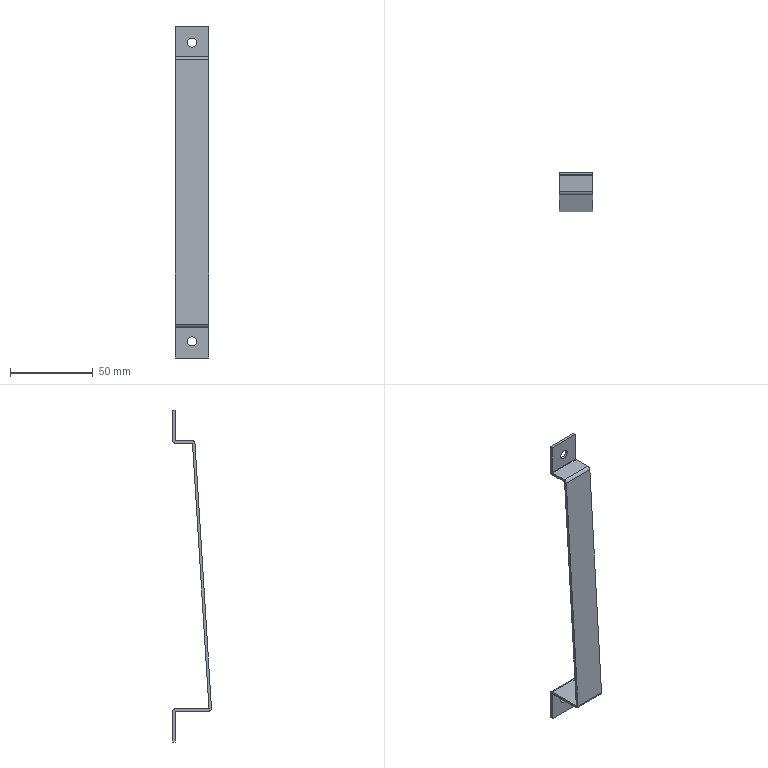Part | SolidWorks | features BaseBody 1, ICE 1 | 1 solid | 26 faces | box 20 x 23.481 x 200 mm | volume 6904 mm3 | plane 14 | cylinder 12 | commonest cylinder face diameters 0.6 x4 3.6 x4 5.5 x4
STEP:
#1=CARTESIAN_POINT('',(-17.75,-8.,134.));
#2=VERTEX_POINT('',#1);
#3=CARTESIAN_POINT('',(-23.25,-8.,134.));
#4=VERTEX_POINT('',#3);
#5=CARTESIAN_POINT('',(-20.5,-8.,134.));
#6=DIRECTION('',(0.,1.,0.));
#7=DIRECTION('',(-1.,0.,0.));
#8=AXIS2_PLACEMENT_3D('',#5,#6,#7);
#9=CIRCLE('',#8,2.75);
#10=EDGE_CURVE('',#2,#4,#9,.T.);
#11=ORIENTED_EDGE('',*,*,#10,.F.);
#12=CARTESIAN_POINT('',(-17.75,-6.5,134.));
#13=VERTEX_POINT('',#12);
#14=CARTESIAN_POINT('',(-17.75,-29.981,134.));
#15=DIRECTION('',(0.,1.,0.));
#16=VECTOR('',#15,1000.);
#17=LINE('',#14,#16);
#18=EDGE_CURVE('',#2,#13,#17,.T.);
#19=ORIENTED_EDGE('',*,*,#18,.T.);
#20=CARTESIAN_POINT('',(-23.25,-6.5,134.));
#21=VERTEX_POINT('',#20);
#22=CARTESIAN_POINT('',(-20.5,-6.5,134.));
#23=DIRECTION('',(0.,1.,0.));
#24=DIRECTION('',(-1.,0.,0.));
#25=AXIS2_PLACEMENT_3D('',#22,#23,#24);
#26=CIRCLE('',#25,2.75);
#27=EDGE_CURVE('',#13,#21,#26,.T.);
#28=ORIENTED_EDGE('',*,*,#27,.T.);
#29=CARTESIAN_POINT('',(-23.25,-29.981,134.));
#30=DIRECTION('',(0.,1.,0.));
#31=VECTOR('',#30,1000.);
#32=LINE('',#29,#31);
#33=EDGE_CURVE('',#4,#21,#32,.T.);
#34=ORIENTED_EDGE('',*,*,#33,.F.);
#35=EDGE_LOOP('',(#11,#19,#28,#34));
#36=FACE_OUTER_BOUND('',#35,.T.);
#37=CARTESIAN_POINT('',(-20.5,-29.981,134.));
#38=DIRECTION('',(0.,1.,0.));
#39=DIRECTION('',(-1.,0.,0.));
#40=AXIS2_PLACEMENT_3D('',#37,#38,#39);
#41=CYLINDRICAL_SURFACE('',#40,2.75);
#42=ADVANCED_FACE('',(#36),#41,.F.);
#43=CARTESIAN_POINT('',(-17.75,-8.,-46.));
#44=VERTEX_POINT('',#43);
#45=CARTESIAN_POINT('',(-23.25,-8.,-46.));
#46=VERTEX_POINT('',#45);
#47=CARTESIAN_POINT('',(-20.5,-8.,-46.));
#48=DIRECTION('',(0.,1.,0.));
#49=DIRECTION('',(-1.,0.,0.));
#50=AXIS2_PLACEMENT_3D('',#47,#48,#49);
#51=CIRCLE('',#50,2.75);
#52=EDGE_CURVE('',#44,#46,#51,.T.);
#53=ORIENTED_EDGE('',*,*,#52,.F.);
#54=CARTESIAN_POINT('',(-17.75,-6.5,-46.));
#55=VERTEX_POINT('',#54);
#56=CARTESIAN_POINT('',(-17.75,-29.981,-46.));
#57=DIRECTION('',(0.,1.,0.));
#58=VECTOR('',#57,1000.);
#59=LINE('',#56,#58);
#60=EDGE_CURVE('',#44,#55,#59,.T.);
#61=ORIENTED_EDGE('',*,*,#60,.T.);
#62=CARTESIAN_POINT('',(-23.25,-6.5,-46.));
#63=VERTEX_POINT('',#62);
#64=CARTESIAN_POINT('',(-20.5,-6.5,-46.));
#65=DIRECTION('',(0.,1.,0.));
#66=DIRECTION('',(-1.,0.,0.));
#67=AXIS2_PLACEMENT_3D('',#64,#65,#66);
#68=CIRCLE('',#67,2.75);
#69=EDGE_CURVE('',#55,#63,#68,.T.);
#70=ORIENTED_EDGE('',*,*,#69,.T.);
#71=CARTESIAN_POINT('',(-23.25,-29.981,-46.));
#72=DIRECTION('',(0.,1.,0.));
#73=VECTOR('',#72,1000.);
#74=LINE('',#71,#73);
#75=EDGE_CURVE('',#46,#63,#74,.T.);
#76=ORIENTED_EDGE('',*,*,#75,.F.);
#77=EDGE_LOOP('',(#53,#61,#70,#76));
#78=FACE_OUTER_BOUND('',#77,.T.);
#79=CARTESIAN_POINT('',(-20.5,-29.981,-46.));
#80=DIRECTION('',(0.,1.,0.));
#81=DIRECTION('',(-1.,0.,0.));
#82=AXIS2_PLACEMENT_3D('',#79,#80,#81);
#83=CYLINDRICAL_SURFACE('',#82,2.75);
#84=ADVANCED_FACE('',(#78),#83,.F.);
#85=CARTESIAN_POINT('',(-30.5,-20.015,123.812));
#86=VERTEX_POINT('',#85);
#87=CARTESIAN_POINT('',(-10.5,-20.015,123.812));
#88=VERTEX_POINT('',#87);
#89=CARTESIAN_POINT('',(-30.5,-20.015,123.812));
#90=DIRECTION('',(1.,0.,0.));
#91=VECTOR('',#90,1000.);
#92=LINE('',#89,#91);
#93=EDGE_CURVE('',#86,#88,#92,.T.);
#94=ORIENTED_EDGE('',*,*,#93,.F.);
#95=CARTESIAN_POINT('',(-30.5,-29.977,-35.588));
#96=VERTEX_POINT('',#95);
#97=CARTESIAN_POINT('',(-30.5,-29.997,-35.906));
#98=DIRECTION('',(0.,0.06238,0.9981));
#99=VECTOR('',#98,1000.);
#100=LINE('',#97,#99);
#101=EDGE_CURVE('',#96,#86,#100,.T.);
#102=ORIENTED_EDGE('',*,*,#101,.F.);
#103=CARTESIAN_POINT('',(-10.5,-29.977,-35.588));
#104=VERTEX_POINT('',#103);
#105=CARTESIAN_POINT('',(-30.5,-29.977,-35.588));
#106=DIRECTION('',(-1.,0.,0.));
#107=VECTOR('',#106,1000.);
#108=LINE('',#105,#107);
#109=EDGE_CURVE('',#104,#96,#108,.T.);
#110=ORIENTED_EDGE('',*,*,#109,.F.);
#111=CARTESIAN_POINT('',(-10.5,-29.997,-35.906));
#112=DIRECTION('',(0.,-0.06238,-0.9981));
#113=VECTOR('',#112,1000.);
#114=LINE('',#111,#113);
#115=EDGE_CURVE('',#88,#104,#114,.T.);
#116=ORIENTED_EDGE('',*,*,#115,.F.);
#117=EDGE_LOOP('',(#94,#102,#110,#116));
#118=FACE_OUTER_BOUND('',#117,.T.);
#119=CARTESIAN_POINT('',(-30.5,-29.997,-35.906));
#120=DIRECTION('',(0.,0.9981,-0.06238));
#121=DIRECTION('',(0.,0.06238,0.9981));
#122=AXIS2_PLACEMENT_3D('',#119,#120,#121);
#123=PLANE('',#122);
#124=ADVANCED_FACE('',(#118),#123,.F.);
#125=ORIENTED_EDGE('',*,*,#115,.T.);
#126=CARTESIAN_POINT('',(-10.5,-28.181,-37.5));
#127=VERTEX_POINT('',#126);
#128=CARTESIAN_POINT('',(-10.5,-28.181,-35.7));
#129=DIRECTION('',(-1.,0.,0.));
#130=DIRECTION('',(0.,1.,0.));
#131=AXIS2_PLACEMENT_3D('',#128,#129,#130);
#132=CIRCLE('',#131,1.8);
#133=EDGE_CURVE('',#127,#104,#132,.T.);
#134=ORIENTED_EDGE('',*,*,#133,.F.);
#135=CARTESIAN_POINT('',(-10.5,-8.3,-37.5));
#136=VERTEX_POINT('',#135);
#137=CARTESIAN_POINT('',(-10.5,-6.5,-37.5));
#138=DIRECTION('',(0.,1.,0.));
#139=VECTOR('',#138,1000.);
#140=LINE('',#137,#139);
#141=EDGE_CURVE('',#127,#136,#140,.T.);
#142=ORIENTED_EDGE('',*,*,#141,.T.);
#143=CARTESIAN_POINT('',(-10.5,-8.,-37.8));
#144=VERTEX_POINT('',#143);
#145=CARTESIAN_POINT('',(-10.5,-8.3,-37.8));
#146=DIRECTION('',(-1.,0.,0.));
#147=DIRECTION('',(0.,1.,0.));
#148=AXIS2_PLACEMENT_3D('',#145,#146,#147);
#149=CIRCLE('',#148,0.3);
#150=EDGE_CURVE('',#136,#144,#149,.T.);
#151=ORIENTED_EDGE('',*,*,#150,.T.);
#152=CARTESIAN_POINT('',(-10.5,-8.,-56.));
#153=VERTEX_POINT('',#152);
#154=CARTESIAN_POINT('',(-10.5,-8.,-56.));
#155=DIRECTION('',(0.,0.,-1.));
#156=VECTOR('',#155,1000.);
#157=LINE('',#154,#156);
#158=EDGE_CURVE('',#144,#153,#157,.T.);
#159=ORIENTED_EDGE('',*,*,#158,.T.);
#160=CARTESIAN_POINT('',(-10.5,-6.5,-56.));
#161=VERTEX_POINT('',#160);
#162=CARTESIAN_POINT('',(-10.5,-8.3,-56.));
#163=DIRECTION('',(0.,1.,0.));
#164=VECTOR('',#163,1000.);
#165=LINE('',#162,#164);
#166=EDGE_CURVE('',#153,#161,#165,.T.);
#167=ORIENTED_EDGE('',*,*,#166,.T.);
#168=CARTESIAN_POINT('',(-10.5,-6.5,-37.8));
#169=VERTEX_POINT('',#168);
#170=CARTESIAN_POINT('',(-10.5,-6.5,-37.5));
#171=DIRECTION('',(0.,0.,1.));
#172=VECTOR('',#171,1000.);
#173=LINE('',#170,#172);
#174=EDGE_CURVE('',#161,#169,#173,.T.);
#175=ORIENTED_EDGE('',*,*,#174,.T.);
#176=CARTESIAN_POINT('',(-10.5,-8.3,-36.));
#177=VERTEX_POINT('',#176);
#178=CARTESIAN_POINT('',(-10.5,-8.3,-37.8));
#179=DIRECTION('',(-1.,0.,0.));
#180=DIRECTION('',(0.,1.,0.));
#181=AXIS2_PLACEMENT_3D('',#178,#179,#180);
#182=CIRCLE('',#181,1.8);
#183=EDGE_CURVE('',#177,#169,#182,.T.);
#184=ORIENTED_EDGE('',*,*,#183,.F.);
#185=CARTESIAN_POINT('',(-10.5,-28.181,-36.));
#186=VERTEX_POINT('',#185);
#187=CARTESIAN_POINT('',(-10.5,-29.977,-36.));
#188=DIRECTION('',(0.,-1.,0.));
#189=VECTOR('',#188,1000.);
#190=LINE('',#187,#189);
#191=EDGE_CURVE('',#177,#186,#190,.T.);
#192=ORIENTED_EDGE('',*,*,#191,.T.);
#193=CARTESIAN_POINT('',(-10.5,-28.48,-35.681));
#194=VERTEX_POINT('',#193);
#195=CARTESIAN_POINT('',(-10.5,-28.181,-35.7));
#196=DIRECTION('',(-1.,0.,0.));
#197=DIRECTION('',(0.,1.,0.));
#198=AXIS2_PLACEMENT_3D('',#195,#196,#197);
#199=CIRCLE('',#198,0.3);
#200=EDGE_CURVE('',#186,#194,#199,.T.);
#201=ORIENTED_EDGE('',*,*,#200,.T.);
#202=CARTESIAN_POINT('',(-10.5,-18.518,123.719));
#203=VERTEX_POINT('',#202);
#204=CARTESIAN_POINT('',(-10.5,-28.48,-35.681));
#205=DIRECTION('',(0.,0.06238,0.9981));
#206=VECTOR('',#205,1000.);
#207=LINE('',#204,#206);
#208=EDGE_CURVE('',#194,#203,#207,.T.);
#209=ORIENTED_EDGE('',*,*,#208,.T.);
#210=CARTESIAN_POINT('',(-10.5,-18.218,124.));
#211=VERTEX_POINT('',#210);
#212=CARTESIAN_POINT('',(-10.5,-18.218,123.7));
#213=DIRECTION('',(-1.,0.,0.));
#214=DIRECTION('',(0.,1.,0.));
#215=AXIS2_PLACEMENT_3D('',#212,#213,#214);
#216=CIRCLE('',#215,0.3);
#217=EDGE_CURVE('',#203,#211,#216,.T.);
#218=ORIENTED_EDGE('',*,*,#217,.T.);
#219=CARTESIAN_POINT('',(-10.5,-8.3,124.));
#220=VERTEX_POINT('',#219);
#221=CARTESIAN_POINT('',(-10.5,-8.,124.));
#222=DIRECTION('',(0.,1.,0.));
#223=VECTOR('',#222,1000.);
#224=LINE('',#221,#223);
#225=EDGE_CURVE('',#211,#220,#224,.T.);
#226=ORIENTED_EDGE('',*,*,#225,.T.);
#227=CARTESIAN_POINT('',(-10.5,-6.5,125.8));
#228=VERTEX_POINT('',#227);
#229=CARTESIAN_POINT('',(-10.5,-8.3,125.8));
#230=DIRECTION('',(-1.,0.,0.));
#231=DIRECTION('',(0.,1.,0.));
#232=AXIS2_PLACEMENT_3D('',#229,#230,#231);
#233=CIRCLE('',#232,1.8);
#234=EDGE_CURVE('',#228,#220,#233,.T.);
#235=ORIENTED_EDGE('',*,*,#234,.F.);
#236=CARTESIAN_POINT('',(-10.5,-6.5,144.));
#237=VERTEX_POINT('',#236);
#238=CARTESIAN_POINT('',(-10.5,-6.5,125.8));
#239=DIRECTION('',(0.,0.,-1.));
#240=VECTOR('',#239,1000.);
#241=LINE('',#238,#240);
#242=EDGE_CURVE('',#237,#228,#241,.T.);
#243=ORIENTED_EDGE('',*,*,#242,.F.);
#244=CARTESIAN_POINT('',(-10.5,-8.,144.));
#245=VERTEX_POINT('',#244);
#246=CARTESIAN_POINT('',(-10.5,-8.3,144.));
#247=DIRECTION('',(0.,1.,0.));
#248=VECTOR('',#247,1000.);
#249=LINE('',#246,#248);
#250=EDGE_CURVE('',#245,#237,#249,.T.);
#251=ORIENTED_EDGE('',*,*,#250,.F.);
#252=CARTESIAN_POINT('',(-10.5,-8.,125.8));
#253=VERTEX_POINT('',#252);
#254=CARTESIAN_POINT('',(-10.5,-8.,124.));
#255=DIRECTION('',(0.,0.,-1.));
#256=VECTOR('',#255,1000.);
#257=LINE('',#254,#256);
#258=EDGE_CURVE('',#245,#253,#257,.T.);
#259=ORIENTED_EDGE('',*,*,#258,.T.);
#260=CARTESIAN_POINT('',(-10.5,-8.3,125.5));
#261=VERTEX_POINT('',#260);
#262=CARTESIAN_POINT('',(-10.5,-8.3,125.8));
#263=DIRECTION('',(-1.,0.,0.));
#264=DIRECTION('',(0.,1.,0.));
#265=AXIS2_PLACEMENT_3D('',#262,#263,#264);
#266=CIRCLE('',#265,0.3);
#267=EDGE_CURVE('',#253,#261,#266,.T.);
#268=ORIENTED_EDGE('',*,*,#267,.T.);
#269=CARTESIAN_POINT('',(-10.5,-18.218,125.5));
#270=VERTEX_POINT('',#269);
#271=CARTESIAN_POINT('',(-10.5,-18.5,125.5));
#272=DIRECTION('',(0.,-1.,0.));
#273=VECTOR('',#272,1000.);
#274=LINE('',#271,#273);
#275=EDGE_CURVE('',#261,#270,#274,.T.);
#276=ORIENTED_EDGE('',*,*,#275,.T.);
#277=CARTESIAN_POINT('',(-10.5,-18.218,123.7));
#278=DIRECTION('',(-1.,0.,0.));
#279=DIRECTION('',(0.,1.,0.));
#280=AXIS2_PLACEMENT_3D('',#277,#278,#279);
#281=CIRCLE('',#280,1.8);
#282=EDGE_CURVE('',#88,#270,#281,.T.);
#283=ORIENTED_EDGE('',*,*,#282,.F.);
#284=EDGE_LOOP('',(#125,#134,#142,#151,#159,#167,#175,#184,#192,#201,#209,#218,#226,#235,#243,#251,#259,#268,#276,#283));
#285=FACE_OUTER_BOUND('',#284,.T.);
#286=CARTESIAN_POINT('',(-10.5,-18.218,125.5));
#287=DIRECTION('',(1.,0.,0.));
#288=DIRECTION('',(0.,1.,0.));
#289=AXIS2_PLACEMENT_3D('',#286,#287,#288);
#290=PLANE('',#289);
#291=ADVANCED_FACE('',(#285),#290,.T.);
#292=CARTESIAN_POINT('',(-30.5,-18.218,125.5));
#293=VERTEX_POINT('',#292);
#294=CARTESIAN_POINT('',(-30.5,-18.218,123.7));
#295=DIRECTION('',(1.,0.,0.));
#296=DIRECTION('',(0.,1.,0.));
#297=AXIS2_PLACEMENT_3D('',#294,#295,#296);
#298=CIRCLE('',#297,1.8);
#299=EDGE_CURVE('',#293,#86,#298,.T.);
#300=ORIENTED_EDGE('',*,*,#299,.T.);
#301=ORIENTED_EDGE('',*,*,#93,.T.);
#302=ORIENTED_EDGE('',*,*,#282,.T.);
#303=CARTESIAN_POINT('',(-30.5,-18.218,125.5));
#304=DIRECTION('',(-1.,0.,0.));
#305=VECTOR('',#304,1000.);
#306=LINE('',#303,#305);
#307=EDGE_CURVE('',#270,#293,#306,.T.);
#308=ORIENTED_EDGE('',*,*,#307,.T.);
#309=EDGE_LOOP('',(#300,#301,#302,#308));
#310=FACE_OUTER_BOUND('',#309,.T.);
#311=CARTESIAN_POINT('',(-30.5,-18.218,123.7));
#312=DIRECTION('',(1.,0.,0.));
#313=DIRECTION('',(0.,1.,0.));
#314=AXIS2_PLACEMENT_3D('',#311,#312,#313);
#315=CYLINDRICAL_SURFACE('',#314,1.8);
#316=ADVANCED_FACE('',(#310),#315,.T.);
#317=ORIENTED_EDGE('',*,*,#101,.T.);
#318=ORIENTED_EDGE('',*,*,#299,.F.);
#319=CARTESIAN_POINT('',(-30.5,-8.3,125.5));
#320=VERTEX_POINT('',#319);
#321=CARTESIAN_POINT('',(-30.5,-18.5,125.5));
#322=DIRECTION('',(0.,1.,0.));
#323=VECTOR('',#322,1000.);
#324=LINE('',#321,#323);
#325=EDGE_CURVE('',#293,#320,#324,.T.);
#326=ORIENTED_EDGE('',*,*,#325,.T.);
#327=CARTESIAN_POINT('',(-30.5,-8.,125.8));
#328=VERTEX_POINT('',#327);
#329=CARTESIAN_POINT('',(-30.5,-8.3,125.8));
#330=DIRECTION('',(1.,0.,0.));
#331=DIRECTION('',(0.,1.,0.));
#332=AXIS2_PLACEMENT_3D('',#329,#330,#331);
#333=CIRCLE('',#332,0.3);
#334=EDGE_CURVE('',#320,#328,#333,.T.);
#335=ORIENTED_EDGE('',*,*,#334,.T.);
#336=CARTESIAN_POINT('',(-30.5,-8.,144.));
#337=VERTEX_POINT('',#336);
#338=CARTESIAN_POINT('',(-30.5,-8.,124.));
#339=DIRECTION('',(0.,0.,1.));
#340=VECTOR('',#339,1000.);
#341=LINE('',#338,#340);
#342=EDGE_CURVE('',#328,#337,#341,.T.);
#343=ORIENTED_EDGE('',*,*,#342,.T.);
#344=CARTESIAN_POINT('',(-30.5,-6.5,144.));
#345=VERTEX_POINT('',#344);
#346=CARTESIAN_POINT('',(-30.5,-6.5,144.));
#347=DIRECTION('',(0.,-1.,0.));
#348=VECTOR('',#347,1000.);
#349=LINE('',#346,#348);
#350=EDGE_CURVE('',#345,#337,#349,.T.);
#351=ORIENTED_EDGE('',*,*,#350,.F.);
#352=CARTESIAN_POINT('',(-30.5,-6.5,125.8));
#353=VERTEX_POINT('',#352);
#354=CARTESIAN_POINT('',(-30.5,-6.5,125.5));
#355=DIRECTION('',(0.,0.,-1.));
#356=VECTOR('',#355,1000.);
#357=LINE('',#354,#356);
#358=EDGE_CURVE('',#345,#353,#357,.T.);
#359=ORIENTED_EDGE('',*,*,#358,.T.);
#360=CARTESIAN_POINT('',(-30.5,-8.3,124.));
#361=VERTEX_POINT('',#360);
#362=CARTESIAN_POINT('',(-30.5,-8.3,125.8));
#363=DIRECTION('',(1.,0.,0.));
#364=DIRECTION('',(0.,1.,0.));
#365=AXIS2_PLACEMENT_3D('',#362,#363,#364);
#366=CIRCLE('',#365,1.8);
#367=EDGE_CURVE('',#361,#353,#366,.T.);
#368=ORIENTED_EDGE('',*,*,#367,.F.);
#369=CARTESIAN_POINT('',(-30.5,-18.218,124.));
#370=VERTEX_POINT('',#369);
#371=CARTESIAN_POINT('',(-30.5,-20.015,124.));
#372=DIRECTION('',(0.,-1.,0.));
#373=VECTOR('',#372,1000.);
#374=LINE('',#371,#373);
#375=EDGE_CURVE('',#361,#370,#374,.T.);
#376=ORIENTED_EDGE('',*,*,#375,.T.);
#377=CARTESIAN_POINT('',(-30.5,-18.518,123.719));
#378=VERTEX_POINT('',#377);
#379=CARTESIAN_POINT('',(-30.5,-18.218,123.7));
#380=DIRECTION('',(1.,0.,0.));
#381=DIRECTION('',(0.,1.,0.));
#382=AXIS2_PLACEMENT_3D('',#379,#380,#381);
#383=CIRCLE('',#382,0.3);
#384=EDGE_CURVE('',#370,#378,#383,.T.);
#385=ORIENTED_EDGE('',*,*,#384,.T.);
#386=CARTESIAN_POINT('',(-30.5,-28.48,-35.681));
#387=VERTEX_POINT('',#386);
#388=CARTESIAN_POINT('',(-30.5,-18.518,123.719));
#389=DIRECTION('',(0.,-0.06238,-0.9981));
#390=VECTOR('',#389,1000.);
#391=LINE('',#388,#390);
#392=EDGE_CURVE('',#378,#387,#391,.T.);
#393=ORIENTED_EDGE('',*,*,#392,.T.);
#394=CARTESIAN_POINT('',(-30.5,-28.181,-36.));
#395=VERTEX_POINT('',#394);
#396=CARTESIAN_POINT('',(-30.5,-28.181,-35.7));
#397=DIRECTION('',(1.,0.,0.));
#398=DIRECTION('',(0.,1.,0.));
#399=AXIS2_PLACEMENT_3D('',#396,#397,#398);
#400=CIRCLE('',#399,0.3);
#401=EDGE_CURVE('',#387,#395,#400,.T.);
#402=ORIENTED_EDGE('',*,*,#401,.T.);
#403=CARTESIAN_POINT('',(-30.5,-8.3,-36.));
#404=VERTEX_POINT('',#403);
#405=CARTESIAN_POINT('',(-30.5,-8.,-36.));
#406=DIRECTION('',(0.,1.,0.));
#407=VECTOR('',#406,1000.);
#408=LINE('',#405,#407);
#409=EDGE_CURVE('',#395,#404,#408,.T.);
#410=ORIENTED_EDGE('',*,*,#409,.T.);
#411=CARTESIAN_POINT('',(-30.5,-6.5,-37.8));
#412=VERTEX_POINT('',#411);
#413=CARTESIAN_POINT('',(-30.5,-8.3,-37.8));
#414=DIRECTION('',(1.,0.,0.));
#415=DIRECTION('',(0.,1.,0.));
#416=AXIS2_PLACEMENT_3D('',#413,#414,#415);
#417=CIRCLE('',#416,1.8);
#418=EDGE_CURVE('',#412,#404,#417,.T.);
#419=ORIENTED_EDGE('',*,*,#418,.F.);
#420=CARTESIAN_POINT('',(-30.5,-6.5,-56.));
#421=VERTEX_POINT('',#420);
#422=CARTESIAN_POINT('',(-30.5,-6.5,125.8));
#423=DIRECTION('',(0.,0.,-1.));
#424=VECTOR('',#423,1000.);
#425=LINE('',#422,#424);
#426=EDGE_CURVE('',#412,#421,#425,.T.);
#427=ORIENTED_EDGE('',*,*,#426,.T.);
#428=CARTESIAN_POINT('',(-30.5,-8.,-56.));
#429=VERTEX_POINT('',#428);
#430=CARTESIAN_POINT('',(-30.5,-8.3,-56.));
#431=DIRECTION('',(0.,-1.,0.));
#432=VECTOR('',#431,1000.);
#433=LINE('',#430,#432);
#434=EDGE_CURVE('',#421,#429,#433,.T.);
#435=ORIENTED_EDGE('',*,*,#434,.T.);
#436=CARTESIAN_POINT('',(-30.5,-8.,-37.8));
#437=VERTEX_POINT('',#436);
#438=CARTESIAN_POINT('',(-30.5,-8.,-56.));
#439=DIRECTION('',(0.,0.,1.));
#440=VECTOR('',#439,1000.);
#441=LINE('',#438,#440);
#442=EDGE_CURVE('',#429,#437,#441,.T.);
#443=ORIENTED_EDGE('',*,*,#442,.T.);
#444=CARTESIAN_POINT('',(-30.5,-8.3,-37.5));
#445=VERTEX_POINT('',#444);
#446=CARTESIAN_POINT('',(-30.5,-8.3,-37.8));
#447=DIRECTION('',(1.,0.,0.));
#448=DIRECTION('',(0.,1.,0.));
#449=AXIS2_PLACEMENT_3D('',#446,#447,#448);
#450=CIRCLE('',#449,0.3);
#451=EDGE_CURVE('',#437,#445,#450,.T.);
#452=ORIENTED_EDGE('',*,*,#451,.T.);
#453=CARTESIAN_POINT('',(-30.5,-28.181,-37.5));
#454=VERTEX_POINT('',#453);
#455=CARTESIAN_POINT('',(-30.5,-6.5,-37.5));
#456=DIRECTION('',(0.,-1.,0.));
#457=VECTOR('',#456,1000.);
#458=LINE('',#455,#457);
#459=EDGE_CURVE('',#445,#454,#458,.T.);
#460=ORIENTED_EDGE('',*,*,#459,.T.);
#461=CARTESIAN_POINT('',(-30.5,-28.181,-35.7));
#462=DIRECTION('',(1.,0.,0.));
#463=DIRECTION('',(0.,1.,0.));
#464=AXIS2_PLACEMENT_3D('',#461,#462,#463);
#465=CIRCLE('',#464,1.8);
#466=EDGE_CURVE('',#96,#454,#465,.T.);
#467=ORIENTED_EDGE('',*,*,#466,.F.);
#468=EDGE_LOOP('',(#317,#318,#326,#335,#343,#351,#359,#368,#376,#385,#393,#402,#410,#419,#427,#435,#443,#452,#460,#467));
#469=FACE_OUTER_BOUND('',#468,.T.);
#470=CARTESIAN_POINT('',(-30.5,-28.181,-37.5));
#471=DIRECTION('',(-1.,0.,0.));
#472=DIRECTION('',(0.,-1.,0.));
#473=AXIS2_PLACEMENT_3D('',#470,#471,#472);
#474=PLANE('',#473);
#475=ADVANCED_FACE('',(#469),#474,.T.);
#476=ORIENTED_EDGE('',*,*,#466,.T.);
#477=CARTESIAN_POINT('',(-30.5,-28.181,-37.5));
#478=DIRECTION('',(1.,0.,0.));
#479=VECTOR('',#478,1000.);
#480=LINE('',#477,#479);
#481=EDGE_CURVE('',#454,#127,#480,.T.);
#482=ORIENTED_EDGE('',*,*,#481,.T.);
#483=ORIENTED_EDGE('',*,*,#133,.T.);
#484=ORIENTED_EDGE('',*,*,#109,.T.);
#485=EDGE_LOOP('',(#476,#482,#483,#484));
#486=FACE_OUTER_BOUND('',#485,.T.);
#487=CARTESIAN_POINT('',(-30.5,-28.181,-35.7));
#488=DIRECTION('',(1.,0.,0.));
#489=DIRECTION('',(0.,1.,0.));
#490=AXIS2_PLACEMENT_3D('',#487,#488,#489);
#491=CYLINDRICAL_SURFACE('',#490,1.8);
#492=ADVANCED_FACE('',(#486),#491,.T.);
#493=ORIENTED_EDGE('',*,*,#392,.F.);
#494=CARTESIAN_POINT('',(-30.5,-18.518,123.719));
#495=DIRECTION('',(1.,0.,0.));
#496=VECTOR('',#495,1000.);
#497=LINE('',#494,#496);
#498=EDGE_CURVE('',#378,#203,#497,.T.);
#499=ORIENTED_EDGE('',*,*,#498,.T.);
#500=ORIENTED_EDGE('',*,*,#208,.F.);
#501=CARTESIAN_POINT('',(-30.5,-28.48,-35.681));
#502=DIRECTION('',(-1.,0.,0.));
#503=VECTOR('',#502,1000.);
#504=LINE('',#501,#503);
#505=EDGE_CURVE('',#194,#387,#504,.T.);
#506=ORIENTED_EDGE('',*,*,#505,.T.);
#507=EDGE_LOOP('',(#493,#499,#500,#506));
#508=FACE_OUTER_BOUND('',#507,.T.);
#509=CARTESIAN_POINT('',(-30.5,-28.5,-36.));
#510=DIRECTION('',(0.,0.9981,-0.06238));
#511=DIRECTION('',(0.,0.06238,0.9981));
#512=AXIS2_PLACEMENT_3D('',#509,#510,#511);
#513=PLANE('',#512);
#514=ADVANCED_FACE('',(#508),#513,.T.);
#515=CARTESIAN_POINT('',(-30.5,-8.3,125.5));
#516=DIRECTION('',(1.,0.,0.));
#517=VECTOR('',#516,1000.);
#518=LINE('',#515,#517);
#519=EDGE_CURVE('',#320,#261,#518,.T.);
#520=ORIENTED_EDGE('',*,*,#519,.F.);
#521=ORIENTED_EDGE('',*,*,#325,.F.);
#522=ORIENTED_EDGE('',*,*,#307,.F.);
#523=ORIENTED_EDGE('',*,*,#275,.F.);
#524=EDGE_LOOP('',(#520,#521,#522,#523));
#525=FACE_OUTER_BOUND('',#524,.T.);
#526=CARTESIAN_POINT('',(-30.5,-18.5,125.5));
#527=DIRECTION('',(0.,0.,-1.));
#528=DIRECTION('',(0.,1.,0.));
#529=AXIS2_PLACEMENT_3D('',#526,#527,#528);
#530=PLANE('',#529);
#531=ADVANCED_FACE('',(#525),#530,.F.);
#532=ORIENTED_EDGE('',*,*,#481,.F.);
#533=ORIENTED_EDGE('',*,*,#459,.F.);
#534=CARTESIAN_POINT('',(-30.5,-8.3,-37.5));
#535=DIRECTION('',(-1.,0.,0.));
#536=VECTOR('',#535,1000.);
#537=LINE('',#534,#536);
#538=EDGE_CURVE('',#136,#445,#537,.T.);
#539=ORIENTED_EDGE('',*,*,#538,.F.);
#540=ORIENTED_EDGE('',*,*,#141,.F.);
#541=EDGE_LOOP('',(#532,#533,#539,#540));
#542=FACE_OUTER_BOUND('',#541,.T.);
#543=CARTESIAN_POINT('',(-30.5,-6.5,-37.5));
#544=DIRECTION('',(0.,0.,1.));
#545=DIRECTION('',(1.,0.,0.));
#546=AXIS2_PLACEMENT_3D('',#543,#544,#545);
#547=PLANE('',#546);
#548=ADVANCED_FACE('',(#542),#547,.F.);
#549=ORIENTED_EDGE('',*,*,#498,.F.);
#550=ORIENTED_EDGE('',*,*,#384,.F.);
#551=CARTESIAN_POINT('',(-30.5,-18.218,124.));
#552=DIRECTION('',(-1.,0.,0.));
#553=VECTOR('',#552,1000.);
#554=LINE('',#551,#553);
#555=EDGE_CURVE('',#211,#370,#554,.T.);
#556=ORIENTED_EDGE('',*,*,#555,.F.);
#557=ORIENTED_EDGE('',*,*,#217,.F.);
#558=EDGE_LOOP('',(#549,#550,#556,#557));
#559=FACE_OUTER_BOUND('',#558,.T.);
#560=CARTESIAN_POINT('',(-30.5,-18.218,123.7));
#561=DIRECTION('',(1.,0.,0.));
#562=DIRECTION('',(0.,1.,0.));
#563=AXIS2_PLACEMENT_3D('',#560,#561,#562);
#564=CYLINDRICAL_SURFACE('',#563,0.3);
#565=ADVANCED_FACE('',(#559),#564,.F.);
#566=CARTESIAN_POINT('',(-30.5,-28.181,-36.));
#567=DIRECTION('',(1.,0.,0.));
#568=VECTOR('',#567,1000.);
#569=LINE('',#566,#568);
#570=EDGE_CURVE('',#395,#186,#569,.T.);
#571=ORIENTED_EDGE('',*,*,#570,.F.);
#572=ORIENTED_EDGE('',*,*,#401,.F.);
#573=ORIENTED_EDGE('',*,*,#505,.F.);
#574=ORIENTED_EDGE('',*,*,#200,.F.);
#575=EDGE_LOOP('',(#571,#572,#573,#574));
#576=FACE_OUTER_BOUND('',#575,.T.);
#577=CARTESIAN_POINT('',(-30.5,-28.181,-35.7));
#578=DIRECTION('',(1.,0.,0.));
#579=DIRECTION('',(0.,1.,0.));
#580=AXIS2_PLACEMENT_3D('',#577,#578,#579);
#581=CYLINDRICAL_SURFACE('',#580,0.3);
#582=ADVANCED_FACE('',(#576),#581,.F.);
#583=CARTESIAN_POINT('',(-30.5,-8.,125.8));
#584=DIRECTION('',(1.,0.,0.));
#585=VECTOR('',#584,1000.);
#586=LINE('',#583,#585);
#587=EDGE_CURVE('',#328,#253,#586,.T.);
#588=ORIENTED_EDGE('',*,*,#587,.F.);
#589=ORIENTED_EDGE('',*,*,#334,.F.);
#590=ORIENTED_EDGE('',*,*,#519,.T.);
#591=ORIENTED_EDGE('',*,*,#267,.F.);
#592=EDGE_LOOP('',(#588,#589,#590,#591));
#593=FACE_OUTER_BOUND('',#592,.T.);
#594=CARTESIAN_POINT('',(-30.5,-8.3,125.8));
#595=DIRECTION('',(1.,0.,0.));
#596=DIRECTION('',(0.,1.,0.));
#597=AXIS2_PLACEMENT_3D('',#594,#595,#596);
#598=CYLINDRICAL_SURFACE('',#597,0.3);
#599=ADVANCED_FACE('',(#593),#598,.F.);
#600=ORIENTED_EDGE('',*,*,#538,.T.);
#601=ORIENTED_EDGE('',*,*,#451,.F.);
#602=CARTESIAN_POINT('',(-30.5,-8.,-37.8));
#603=DIRECTION('',(-1.,0.,0.));
#604=VECTOR('',#603,1000.);
#605=LINE('',#602,#604);
#606=EDGE_CURVE('',#144,#437,#605,.T.);
#607=ORIENTED_EDGE('',*,*,#606,.F.);
#608=ORIENTED_EDGE('',*,*,#150,.F.);
#609=EDGE_LOOP('',(#600,#601,#607,#608));
#610=FACE_OUTER_BOUND('',#609,.T.);
#611=CARTESIAN_POINT('',(-30.5,-8.3,-37.8));
#612=DIRECTION('',(1.,0.,0.));
#613=DIRECTION('',(0.,1.,0.));
#614=AXIS2_PLACEMENT_3D('',#611,#612,#613);
#615=CYLINDRICAL_SURFACE('',#614,0.3);
#616=ADVANCED_FACE('',(#610),#615,.F.);
#617=ORIENTED_EDGE('',*,*,#375,.F.);
#618=CARTESIAN_POINT('',(-30.5,-8.3,124.));
#619=DIRECTION('',(1.,0.,0.));
#620=VECTOR('',#619,1000.);
#621=LINE('',#618,#620);
#622=EDGE_CURVE('',#361,#220,#621,.T.);
#623=ORIENTED_EDGE('',*,*,#622,.T.);
#624=ORIENTED_EDGE('',*,*,#225,.F.);
#625=ORIENTED_EDGE('',*,*,#555,.T.);
#626=EDGE_LOOP('',(#617,#623,#624,#625));
#627=FACE_OUTER_BOUND('',#626,.T.);
#628=CARTESIAN_POINT('',(-30.5,-18.5,124.));
#629=DIRECTION('',(0.,0.,-1.));
#630=DIRECTION('',(0.,1.,0.));
#631=AXIS2_PLACEMENT_3D('',#628,#629,#630);
#632=PLANE('',#631);
#633=ADVANCED_FACE('',(#627),#632,.T.);
#634=ORIENTED_EDGE('',*,*,#409,.F.);
#635=ORIENTED_EDGE('',*,*,#570,.T.);
#636=ORIENTED_EDGE('',*,*,#191,.F.);
#637=CARTESIAN_POINT('',(-30.5,-8.3,-36.));
#638=DIRECTION('',(-1.,0.,0.));
#639=VECTOR('',#638,1000.);
#640=LINE('',#637,#639);
#641=EDGE_CURVE('',#177,#404,#640,.T.);
#642=ORIENTED_EDGE('',*,*,#641,.T.);
#643=EDGE_LOOP('',(#634,#635,#636,#642));
#644=FACE_OUTER_BOUND('',#643,.T.);
#645=CARTESIAN_POINT('',(-30.5,-6.5,-36.));
#646=DIRECTION('',(0.,0.,1.));
#647=DIRECTION('',(1.,0.,0.));
#648=AXIS2_PLACEMENT_3D('',#645,#646,#647);
#649=PLANE('',#648);
#650=ADVANCED_FACE('',(#644),#649,.T.);
#651=CARTESIAN_POINT('',(-20.5,-8.,134.));
#652=DIRECTION('',(0.,1.,0.));
#653=DIRECTION('',(-1.,0.,0.));
#654=AXIS2_PLACEMENT_3D('',#651,#652,#653);
#655=CIRCLE('',#654,2.75);
#656=EDGE_CURVE('',#4,#2,#655,.T.);
#657=ORIENTED_EDGE('',*,*,#656,.T.);
#658=ORIENTED_EDGE('',*,*,#10,.T.);
#659=EDGE_LOOP('',(#657,#658));
#660=FACE_BOUND('',#659,.T.);
#661=CARTESIAN_POINT('',(-30.5,-8.,144.));
#662=DIRECTION('',(1.,0.,0.));
#663=VECTOR('',#662,1000.);
#664=LINE('',#661,#663);
#665=EDGE_CURVE('',#337,#245,#664,.T.);
#666=ORIENTED_EDGE('',*,*,#665,.F.);
#667=ORIENTED_EDGE('',*,*,#342,.F.);
#668=ORIENTED_EDGE('',*,*,#587,.T.);
#669=ORIENTED_EDGE('',*,*,#258,.F.);
#670=EDGE_LOOP('',(#666,#667,#668,#669));
#671=FACE_OUTER_BOUND('',#670,.T.);
#672=CARTESIAN_POINT('',(-30.5,-8.,124.));
#673=DIRECTION('',(0.,1.,0.));
#674=DIRECTION('',(-1.,0.,0.));
#675=AXIS2_PLACEMENT_3D('',#672,#673,#674);
#676=PLANE('',#675);
#677=ADVANCED_FACE('',(#660,#671),#676,.F.);
#678=CARTESIAN_POINT('',(-20.5,-8.,-46.));
#679=DIRECTION('',(0.,1.,0.));
#680=DIRECTION('',(-1.,0.,0.));
#681=AXIS2_PLACEMENT_3D('',#678,#679,#680);
#682=CIRCLE('',#681,2.75);
#683=EDGE_CURVE('',#46,#44,#682,.T.);
#684=ORIENTED_EDGE('',*,*,#683,.T.);
#685=ORIENTED_EDGE('',*,*,#52,.T.);
#686=EDGE_LOOP('',(#684,#685));
#687=FACE_BOUND('',#686,.T.);
#688=ORIENTED_EDGE('',*,*,#606,.T.);
#689=ORIENTED_EDGE('',*,*,#442,.F.);
#690=CARTESIAN_POINT('',(-30.5,-8.,-56.));
#691=DIRECTION('',(-1.,0.,0.));
#692=VECTOR('',#691,1000.);
#693=LINE('',#690,#692);
#694=EDGE_CURVE('',#153,#429,#693,.T.);
#695=ORIENTED_EDGE('',*,*,#694,.F.);
#696=ORIENTED_EDGE('',*,*,#158,.F.);
#697=EDGE_LOOP('',(#688,#689,#695,#696));
#698=FACE_OUTER_BOUND('',#697,.T.);
#699=CARTESIAN_POINT('',(-30.5,-8.,-56.));
#700=DIRECTION('',(0.,1.,0.));
#701=DIRECTION('',(-1.,0.,0.));
#702=AXIS2_PLACEMENT_3D('',#699,#700,#701);
#703=PLANE('',#702);
#704=ADVANCED_FACE('',(#687,#698),#703,.F.);
#705=ORIENTED_EDGE('',*,*,#367,.T.);
#706=CARTESIAN_POINT('',(-30.5,-6.5,125.8));
#707=DIRECTION('',(1.,0.,0.));
#708=VECTOR('',#707,1000.);
#709=LINE('',#706,#708);
#710=EDGE_CURVE('',#353,#228,#709,.T.);
#711=ORIENTED_EDGE('',*,*,#710,.T.);
#712=ORIENTED_EDGE('',*,*,#234,.T.);
#713=ORIENTED_EDGE('',*,*,#622,.F.);
#714=EDGE_LOOP('',(#705,#711,#712,#713));
#715=FACE_OUTER_BOUND('',#714,.T.);
#716=CARTESIAN_POINT('',(-30.5,-8.3,125.8));
#717=DIRECTION('',(1.,0.,0.));
#718=DIRECTION('',(0.,1.,0.));
#719=AXIS2_PLACEMENT_3D('',#716,#717,#718);
#720=CYLINDRICAL_SURFACE('',#719,1.8);
#721=ADVANCED_FACE('',(#715),#720,.T.);
#722=ORIENTED_EDGE('',*,*,#418,.T.);
#723=ORIENTED_EDGE('',*,*,#641,.F.);
#724=ORIENTED_EDGE('',*,*,#183,.T.);
#725=CARTESIAN_POINT('',(-30.5,-6.5,-37.8));
#726=DIRECTION('',(-1.,0.,0.));
#727=VECTOR('',#726,1000.);
#728=LINE('',#725,#727);
#729=EDGE_CURVE('',#169,#412,#728,.T.);
#730=ORIENTED_EDGE('',*,*,#729,.T.);
#731=EDGE_LOOP('',(#722,#723,#724,#730));
#732=FACE_OUTER_BOUND('',#731,.T.);
#733=CARTESIAN_POINT('',(-30.5,-8.3,-37.8));
#734=DIRECTION('',(1.,0.,0.));
#735=DIRECTION('',(0.,1.,0.));
#736=AXIS2_PLACEMENT_3D('',#733,#734,#735);
#737=CYLINDRICAL_SURFACE('',#736,1.8);
#738=ADVANCED_FACE('',(#732),#737,.T.);
#739=ORIENTED_EDGE('',*,*,#350,.T.);
#740=ORIENTED_EDGE('',*,*,#665,.T.);
#741=ORIENTED_EDGE('',*,*,#250,.T.);
#742=CARTESIAN_POINT('',(-30.5,-6.5,144.));
#743=DIRECTION('',(-1.,0.,0.));
#744=VECTOR('',#743,1000.);
#745=LINE('',#742,#744);
#746=EDGE_CURVE('',#237,#345,#745,.T.);
#747=ORIENTED_EDGE('',*,*,#746,.T.);
#748=EDGE_LOOP('',(#739,#740,#741,#747));
#749=FACE_OUTER_BOUND('',#748,.T.);
#750=CARTESIAN_POINT('',(-30.5,-6.5,144.));
#751=DIRECTION('',(0.,0.,1.));
#752=DIRECTION('',(1.,0.,0.));
#753=AXIS2_PLACEMENT_3D('',#750,#751,#752);
#754=PLANE('',#753);
#755=ADVANCED_FACE('',(#749),#754,.T.);
#756=ORIENTED_EDGE('',*,*,#434,.F.);
#757=CARTESIAN_POINT('',(-30.5,-6.5,-56.));
#758=DIRECTION('',(1.,0.,0.));
#759=VECTOR('',#758,1000.);
#760=LINE('',#757,#759);
#761=EDGE_CURVE('',#421,#161,#760,.T.);
#762=ORIENTED_EDGE('',*,*,#761,.T.);
#763=ORIENTED_EDGE('',*,*,#166,.F.);
#764=ORIENTED_EDGE('',*,*,#694,.T.);
#765=EDGE_LOOP('',(#756,#762,#763,#764));
#766=FACE_OUTER_BOUND('',#765,.T.);
#767=CARTESIAN_POINT('',(-30.5,-8.,-56.));
#768=DIRECTION('',(0.,0.,-1.));
#769=DIRECTION('',(-1.,0.,0.));
#770=AXIS2_PLACEMENT_3D('',#767,#768,#769);
#771=PLANE('',#770);
#772=ADVANCED_FACE('',(#766),#771,.T.);
#773=CARTESIAN_POINT('',(-20.5,-6.5,134.));
#774=DIRECTION('',(0.,1.,0.));
#775=DIRECTION('',(-1.,0.,0.));
#776=AXIS2_PLACEMENT_3D('',#773,#774,#775);
#777=CIRCLE('',#776,2.75);
#778=EDGE_CURVE('',#21,#13,#777,.T.);
#779=ORIENTED_EDGE('',*,*,#778,.F.);
#780=ORIENTED_EDGE('',*,*,#27,.F.);
#781=EDGE_LOOP('',(#779,#780));
#782=FACE_BOUND('',#781,.T.);
#783=ORIENTED_EDGE('',*,*,#358,.F.);
#784=ORIENTED_EDGE('',*,*,#746,.F.);
#785=ORIENTED_EDGE('',*,*,#242,.T.);
#786=ORIENTED_EDGE('',*,*,#710,.F.);
#787=EDGE_LOOP('',(#783,#784,#785,#786));
#788=FACE_OUTER_BOUND('',#787,.T.);
#789=CARTESIAN_POINT('',(-30.5,-6.5,124.));
#790=DIRECTION('',(0.,1.,0.));
#791=DIRECTION('',(-1.,0.,0.));
#792=AXIS2_PLACEMENT_3D('',#789,#790,#791);
#793=PLANE('',#792);
#794=ADVANCED_FACE('',(#782,#788),#793,.T.);
#795=CARTESIAN_POINT('',(-20.5,-6.5,-46.));
#796=DIRECTION('',(0.,1.,0.));
#797=DIRECTION('',(-1.,0.,0.));
#798=AXIS2_PLACEMENT_3D('',#795,#796,#797);
#799=CIRCLE('',#798,2.75);
#800=EDGE_CURVE('',#63,#55,#799,.T.);
#801=ORIENTED_EDGE('',*,*,#800,.F.);
#802=ORIENTED_EDGE('',*,*,#69,.F.);
#803=EDGE_LOOP('',(#801,#802));
#804=FACE_BOUND('',#803,.T.);
#805=ORIENTED_EDGE('',*,*,#426,.F.);
#806=ORIENTED_EDGE('',*,*,#729,.F.);
#807=ORIENTED_EDGE('',*,*,#174,.F.);
#808=ORIENTED_EDGE('',*,*,#761,.F.);
#809=EDGE_LOOP('',(#805,#806,#807,#808));
#810=FACE_OUTER_BOUND('',#809,.T.);
#811=CARTESIAN_POINT('',(-30.5,-6.5,-56.));
#812=DIRECTION('',(0.,1.,0.));
#813=DIRECTION('',(-1.,0.,0.));
#814=AXIS2_PLACEMENT_3D('',#811,#812,#813);
#815=PLANE('',#814);
#816=ADVANCED_FACE('',(#804,#810),#815,.T.);
#817=ORIENTED_EDGE('',*,*,#60,.F.);
#818=ORIENTED_EDGE('',*,*,#683,.F.);
#819=ORIENTED_EDGE('',*,*,#75,.T.);
#820=ORIENTED_EDGE('',*,*,#800,.T.);
#821=EDGE_LOOP('',(#817,#818,#819,#820));
#822=FACE_OUTER_BOUND('',#821,.T.);
#823=CARTESIAN_POINT('',(-20.5,-29.981,-46.));
#824=DIRECTION('',(0.,1.,0.));
#825=DIRECTION('',(-1.,0.,0.));
#826=AXIS2_PLACEMENT_3D('',#823,#824,#825);
#827=CYLINDRICAL_SURFACE('',#826,2.75);
#828=ADVANCED_FACE('',(#822),#827,.F.);
#829=ORIENTED_EDGE('',*,*,#18,.F.);
#830=ORIENTED_EDGE('',*,*,#656,.F.);
#831=ORIENTED_EDGE('',*,*,#33,.T.);
#832=ORIENTED_EDGE('',*,*,#778,.T.);
#833=EDGE_LOOP('',(#829,#830,#831,#832));
#834=FACE_OUTER_BOUND('',#833,.T.);
#835=CARTESIAN_POINT('',(-20.5,-29.981,134.));
#836=DIRECTION('',(0.,1.,0.));
#837=DIRECTION('',(-1.,0.,0.));
#838=AXIS2_PLACEMENT_3D('',#835,#836,#837);
#839=CYLINDRICAL_SURFACE('',#838,2.75);
#840=ADVANCED_FACE('',(#834),#839,.F.);
#841=CLOSED_SHELL('',(#42,#84,#124,#291,#316,#475,#492,#514,#531,#548,#565,#582,#599,#616,#633,#650,#677,#704,#721,#738,#755,#772,#794,#816,#828,#840));
#842=MANIFOLD_SOLID_BREP('',#841);
#843=CARTESIAN_POINT('',(0.,0.,0.));
#844=DIRECTION('',(0.,0.,1.));
#845=DIRECTION('',(1.,0.,0.));
#846=AXIS2_PLACEMENT_3D('',#843,#844,#845);
#847=(LENGTH_UNIT()NAMED_UNIT(*)SI_UNIT(.MILLI.,.METRE.));
#848=UNCERTAINTY_MEASURE_WITH_UNIT(LENGTH_MEASURE(0.00001),#847,'','');
#849=(NAMED_UNIT(*)PLANE_ANGLE_UNIT()SI_UNIT($,.RADIAN.));
#850=(NAMED_UNIT(*)SI_UNIT($,.STERADIAN.)SOLID_ANGLE_UNIT());
#851=(GEOMETRIC_REPRESENTATION_CONTEXT(3)GLOBAL_UNCERTAINTY_ASSIGNED_CONTEXT((#848))GLOBAL_UNIT_ASSIGNED_CONTEXT((#847,#849,#850))REPRESENTATION_CONTEXT('',''));
#852=ADVANCED_BREP_SHAPE_REPRESENTATION('',(#842,#846),#851);